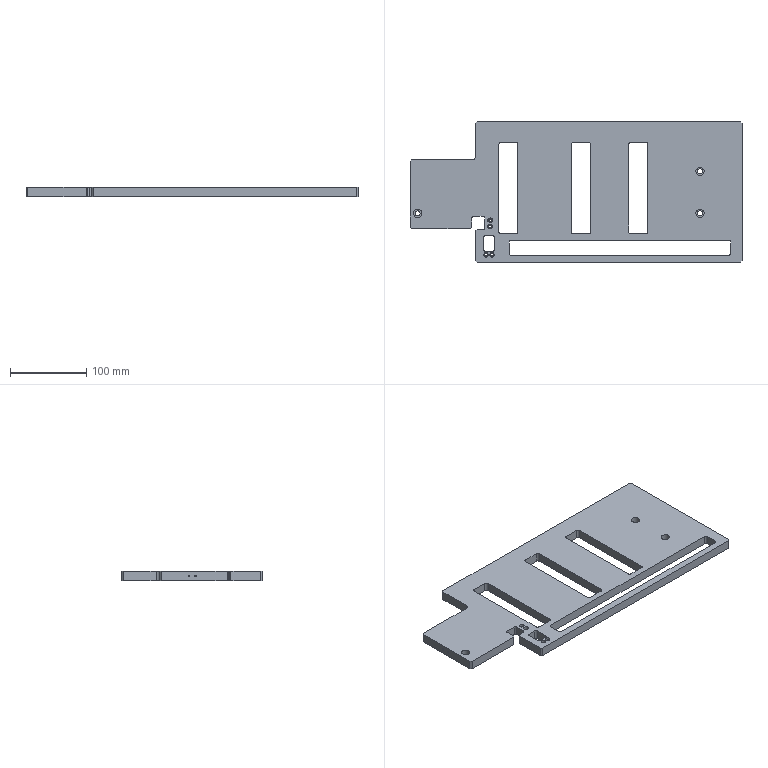Part | 1 solid | 95 faces | box 435 x 184 x 12 mm | volume 675685 mm3 | plane 49 | cylinder 42 | cone 4 | commonest cylinder face diameters 5 x16 6 x8 3.5 x4 4 x3 6.5 x3 11 x3